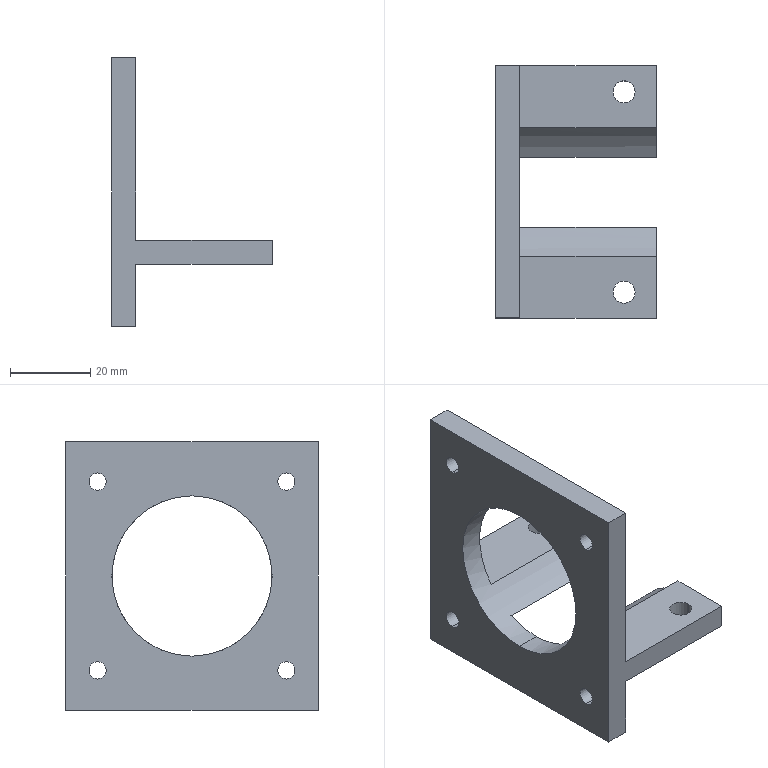Part | SolidWorks | features BaseBody 1 | 1 solid | 27 faces | box 40 x 63 x 67 mm | volume 24720 mm3 | cylinder 14 | plane 13 | commonest cylinder face diameters 4.3 x8 5.5 x4 40 x2
STEP:
#1=CARTESIAN_POINT('',(0.,-23.57,39.42));
#2=VERTEX_POINT('',#1);
#3=CARTESIAN_POINT('',(0.,-23.57,43.72));
#4=VERTEX_POINT('',#3);
#5=CARTESIAN_POINT('',(0.,-23.57,41.57));
#6=DIRECTION('',(-1.,0.,0.));
#7=DIRECTION('',(0.,0.,-1.));
#8=AXIS2_PLACEMENT_3D('',#5,#6,#7);
#9=CIRCLE('',#8,2.15);
#10=EDGE_CURVE('',#2,#4,#9,.T.);
#11=ORIENTED_EDGE('',*,*,#10,.T.);
#12=CARTESIAN_POINT('',(6.,-23.57,43.72));
#13=VERTEX_POINT('',#12);
#14=CARTESIAN_POINT('',(-6.2,-23.57,43.72));
#15=DIRECTION('',(1.,0.,0.));
#16=VECTOR('',#15,1000.);
#17=LINE('',#14,#16);
#18=EDGE_CURVE('',#4,#13,#17,.T.);
#19=ORIENTED_EDGE('',*,*,#18,.T.);
#20=CARTESIAN_POINT('',(6.,-23.57,39.42));
#21=VERTEX_POINT('',#20);
#22=CARTESIAN_POINT('',(6.,-23.57,41.57));
#23=DIRECTION('',(-1.,0.,0.));
#24=DIRECTION('',(0.,0.,-1.));
#25=AXIS2_PLACEMENT_3D('',#22,#23,#24);
#26=CIRCLE('',#25,2.15);
#27=EDGE_CURVE('',#21,#13,#26,.T.);
#28=ORIENTED_EDGE('',*,*,#27,.F.);
#29=CARTESIAN_POINT('',(-6.2,-23.57,39.42));
#30=DIRECTION('',(1.,0.,0.));
#31=VECTOR('',#30,1000.);
#32=LINE('',#29,#31);
#33=EDGE_CURVE('',#2,#21,#32,.T.);
#34=ORIENTED_EDGE('',*,*,#33,.F.);
#35=EDGE_LOOP('',(#11,#19,#28,#34));
#36=FACE_OUTER_BOUND('',#35,.T.);
#37=CARTESIAN_POINT('',(-6.2,-23.57,41.57));
#38=DIRECTION('',(1.,0.,0.));
#39=DIRECTION('',(0.,0.,-1.));
#40=AXIS2_PLACEMENT_3D('',#37,#38,#39);
#41=CYLINDRICAL_SURFACE('',#40,2.15);
#42=ADVANCED_FACE('',(#36),#41,.F.);
#43=CARTESIAN_POINT('',(0.,-23.57,-7.72));
#44=VERTEX_POINT('',#43);
#45=CARTESIAN_POINT('',(0.,-23.57,-3.42));
#46=VERTEX_POINT('',#45);
#47=CARTESIAN_POINT('',(0.,-23.57,-5.57));
#48=DIRECTION('',(-1.,0.,0.));
#49=DIRECTION('',(0.,0.,-1.));
#50=AXIS2_PLACEMENT_3D('',#47,#48,#49);
#51=CIRCLE('',#50,2.15);
#52=EDGE_CURVE('',#44,#46,#51,.T.);
#53=ORIENTED_EDGE('',*,*,#52,.T.);
#54=CARTESIAN_POINT('',(6.,-23.57,-3.42));
#55=VERTEX_POINT('',#54);
#56=CARTESIAN_POINT('',(-6.2,-23.57,-3.42));
#57=DIRECTION('',(1.,0.,0.));
#58=VECTOR('',#57,1000.);
#59=LINE('',#56,#58);
#60=EDGE_CURVE('',#46,#55,#59,.T.);
#61=ORIENTED_EDGE('',*,*,#60,.T.);
#62=CARTESIAN_POINT('',(6.,-23.57,-7.72));
#63=VERTEX_POINT('',#62);
#64=CARTESIAN_POINT('',(6.,-23.57,-5.57));
#65=DIRECTION('',(-1.,0.,0.));
#66=DIRECTION('',(0.,0.,-1.));
#67=AXIS2_PLACEMENT_3D('',#64,#65,#66);
#68=CIRCLE('',#67,2.15);
#69=EDGE_CURVE('',#63,#55,#68,.T.);
#70=ORIENTED_EDGE('',*,*,#69,.F.);
#71=CARTESIAN_POINT('',(-6.2,-23.57,-7.72));
#72=DIRECTION('',(1.,0.,0.));
#73=VECTOR('',#72,1000.);
#74=LINE('',#71,#73);
#75=EDGE_CURVE('',#44,#63,#74,.T.);
#76=ORIENTED_EDGE('',*,*,#75,.F.);
#77=EDGE_LOOP('',(#53,#61,#70,#76));
#78=FACE_OUTER_BOUND('',#77,.T.);
#79=CARTESIAN_POINT('',(-6.2,-23.57,-5.57));
#80=DIRECTION('',(1.,0.,0.));
#81=DIRECTION('',(0.,0.,-1.));
#82=AXIS2_PLACEMENT_3D('',#79,#80,#81);
#83=CYLINDRICAL_SURFACE('',#82,2.15);
#84=ADVANCED_FACE('',(#78),#83,.F.);
#85=CARTESIAN_POINT('',(0.,0.,-2.));
#86=VERTEX_POINT('',#85);
#87=CARTESIAN_POINT('',(0.,0.,38.));
#88=VERTEX_POINT('',#87);
#89=CARTESIAN_POINT('',(0.,0.,18.));
#90=DIRECTION('',(-1.,0.,0.));
#91=DIRECTION('',(0.,0.,-1.));
#92=AXIS2_PLACEMENT_3D('',#89,#90,#91);
#93=CIRCLE('',#92,20.);
#94=EDGE_CURVE('',#86,#88,#93,.T.);
#95=ORIENTED_EDGE('',*,*,#94,.T.);
#96=CARTESIAN_POINT('',(6.,0.,38.));
#97=VERTEX_POINT('',#96);
#98=CARTESIAN_POINT('',(-2.,0.,38.));
#99=DIRECTION('',(1.,0.,0.));
#100=VECTOR('',#99,1000.);
#101=LINE('',#98,#100);
#102=EDGE_CURVE('',#88,#97,#101,.T.);
#103=ORIENTED_EDGE('',*,*,#102,.T.);
#104=CARTESIAN_POINT('',(6.,-16.,6.));
#105=VERTEX_POINT('',#104);
#106=CARTESIAN_POINT('',(6.,0.,18.));
#107=DIRECTION('',(-1.,0.,0.));
#108=DIRECTION('',(0.,0.,-1.));
#109=AXIS2_PLACEMENT_3D('',#106,#107,#108);
#110=CIRCLE('',#109,20.);
#111=EDGE_CURVE('',#105,#97,#110,.T.);
#112=ORIENTED_EDGE('',*,*,#111,.F.);
#113=CARTESIAN_POINT('',(40.,-16.,6.));
#114=VERTEX_POINT('',#113);
#115=CARTESIAN_POINT('',(-2.,-16.,6.));
#116=DIRECTION('',(-1.,0.,0.));
#117=VECTOR('',#116,1000.);
#118=LINE('',#115,#117);
#119=EDGE_CURVE('',#114,#105,#118,.T.);
#120=ORIENTED_EDGE('',*,*,#119,.F.);
#121=CARTESIAN_POINT('',(40.,-8.718,0.));
#122=VERTEX_POINT('',#121);
#123=CARTESIAN_POINT('',(40.,0.,18.));
#124=DIRECTION('',(-1.,0.,0.));
#125=DIRECTION('',(0.,0.,-1.));
#126=AXIS2_PLACEMENT_3D('',#123,#124,#125);
#127=CIRCLE('',#126,20.);
#128=EDGE_CURVE('',#122,#114,#127,.T.);
#129=ORIENTED_EDGE('',*,*,#128,.F.);
#130=CARTESIAN_POINT('',(6.,-8.718,0.));
#131=VERTEX_POINT('',#130);
#132=CARTESIAN_POINT('',(-2.,-8.718,0.));
#133=DIRECTION('',(1.,0.,0.));
#134=VECTOR('',#133,1000.);
#135=LINE('',#132,#134);
#136=EDGE_CURVE('',#131,#122,#135,.T.);
#137=ORIENTED_EDGE('',*,*,#136,.F.);
#138=CARTESIAN_POINT('',(6.,0.,-2.));
#139=VERTEX_POINT('',#138);
#140=CARTESIAN_POINT('',(6.,0.,18.));
#141=DIRECTION('',(-1.,0.,0.));
#142=DIRECTION('',(0.,0.,-1.));
#143=AXIS2_PLACEMENT_3D('',#140,#141,#142);
#144=CIRCLE('',#143,20.);
#145=EDGE_CURVE('',#139,#131,#144,.T.);
#146=ORIENTED_EDGE('',*,*,#145,.F.);
#147=CARTESIAN_POINT('',(-2.,0.,-2.));
#148=DIRECTION('',(1.,0.,0.));
#149=VECTOR('',#148,1000.);
#150=LINE('',#147,#149);
#151=EDGE_CURVE('',#86,#139,#150,.T.);
#152=ORIENTED_EDGE('',*,*,#151,.F.);
#153=EDGE_LOOP('',(#95,#103,#112,#120,#129,#137,#146,#152));
#154=FACE_OUTER_BOUND('',#153,.T.);
#155=CARTESIAN_POINT('',(-2.,0.,18.));
#156=DIRECTION('',(1.,0.,0.));
#157=DIRECTION('',(0.,0.,-1.));
#158=AXIS2_PLACEMENT_3D('',#155,#156,#157);
#159=CYLINDRICAL_SURFACE('',#158,20.);
#160=ADVANCED_FACE('',(#154),#159,.F.);
#161=CARTESIAN_POINT('',(0.,23.57,39.42));
#162=VERTEX_POINT('',#161);
#163=CARTESIAN_POINT('',(0.,23.57,43.72));
#164=VERTEX_POINT('',#163);
#165=CARTESIAN_POINT('',(0.,23.57,41.57));
#166=DIRECTION('',(-1.,0.,0.));
#167=DIRECTION('',(0.,0.,-1.));
#168=AXIS2_PLACEMENT_3D('',#165,#166,#167);
#169=CIRCLE('',#168,2.15);
#170=EDGE_CURVE('',#162,#164,#169,.T.);
#171=ORIENTED_EDGE('',*,*,#170,.T.);
#172=CARTESIAN_POINT('',(6.,23.57,43.72));
#173=VERTEX_POINT('',#172);
#174=CARTESIAN_POINT('',(-6.2,23.57,43.72));
#175=DIRECTION('',(1.,0.,0.));
#176=VECTOR('',#175,1000.);
#177=LINE('',#174,#176);
#178=EDGE_CURVE('',#164,#173,#177,.T.);
#179=ORIENTED_EDGE('',*,*,#178,.T.);
#180=CARTESIAN_POINT('',(6.,23.57,39.42));
#181=VERTEX_POINT('',#180);
#182=CARTESIAN_POINT('',(6.,23.57,41.57));
#183=DIRECTION('',(-1.,0.,0.));
#184=DIRECTION('',(0.,0.,-1.));
#185=AXIS2_PLACEMENT_3D('',#182,#183,#184);
#186=CIRCLE('',#185,2.15);
#187=EDGE_CURVE('',#181,#173,#186,.T.);
#188=ORIENTED_EDGE('',*,*,#187,.F.);
#189=CARTESIAN_POINT('',(-6.2,23.57,39.42));
#190=DIRECTION('',(1.,0.,0.));
#191=VECTOR('',#190,1000.);
#192=LINE('',#189,#191);
#193=EDGE_CURVE('',#162,#181,#192,.T.);
#194=ORIENTED_EDGE('',*,*,#193,.F.);
#195=EDGE_LOOP('',(#171,#179,#188,#194));
#196=FACE_OUTER_BOUND('',#195,.T.);
#197=CARTESIAN_POINT('',(-6.2,23.57,41.57));
#198=DIRECTION('',(1.,0.,0.));
#199=DIRECTION('',(0.,0.,-1.));
#200=AXIS2_PLACEMENT_3D('',#197,#198,#199);
#201=CYLINDRICAL_SURFACE('',#200,2.15);
#202=ADVANCED_FACE('',(#196),#201,.F.);
#203=CARTESIAN_POINT('',(0.,23.57,-7.72));
#204=VERTEX_POINT('',#203);
#205=CARTESIAN_POINT('',(0.,23.57,-3.42));
#206=VERTEX_POINT('',#205);
#207=CARTESIAN_POINT('',(0.,23.57,-5.57));
#208=DIRECTION('',(-1.,0.,0.));
#209=DIRECTION('',(0.,0.,-1.));
#210=AXIS2_PLACEMENT_3D('',#207,#208,#209);
#211=CIRCLE('',#210,2.15);
#212=EDGE_CURVE('',#204,#206,#211,.T.);
#213=ORIENTED_EDGE('',*,*,#212,.T.);
#214=CARTESIAN_POINT('',(6.,23.57,-3.42));
#215=VERTEX_POINT('',#214);
#216=CARTESIAN_POINT('',(-6.2,23.57,-3.42));
#217=DIRECTION('',(1.,0.,0.));
#218=VECTOR('',#217,1000.);
#219=LINE('',#216,#218);
#220=EDGE_CURVE('',#206,#215,#219,.T.);
#221=ORIENTED_EDGE('',*,*,#220,.T.);
#222=CARTESIAN_POINT('',(6.,23.57,-7.72));
#223=VERTEX_POINT('',#222);
#224=CARTESIAN_POINT('',(6.,23.57,-5.57));
#225=DIRECTION('',(-1.,0.,0.));
#226=DIRECTION('',(0.,0.,-1.));
#227=AXIS2_PLACEMENT_3D('',#224,#225,#226);
#228=CIRCLE('',#227,2.15);
#229=EDGE_CURVE('',#223,#215,#228,.T.);
#230=ORIENTED_EDGE('',*,*,#229,.F.);
#231=CARTESIAN_POINT('',(-6.2,23.57,-7.72));
#232=DIRECTION('',(1.,0.,0.));
#233=VECTOR('',#232,1000.);
#234=LINE('',#231,#233);
#235=EDGE_CURVE('',#204,#223,#234,.T.);
#236=ORIENTED_EDGE('',*,*,#235,.F.);
#237=EDGE_LOOP('',(#213,#221,#230,#236));
#238=FACE_OUTER_BOUND('',#237,.T.);
#239=CARTESIAN_POINT('',(-6.2,23.57,-5.57));
#240=DIRECTION('',(1.,0.,0.));
#241=DIRECTION('',(0.,0.,-1.));
#242=AXIS2_PLACEMENT_3D('',#239,#240,#241);
#243=CYLINDRICAL_SURFACE('',#242,2.15);
#244=ADVANCED_FACE('',(#238),#243,.F.);
#245=CARTESIAN_POINT('',(34.75,25.,0.));
#246=VERTEX_POINT('',#245);
#247=CARTESIAN_POINT('',(29.25,25.,0.));
#248=VERTEX_POINT('',#247);
#249=CARTESIAN_POINT('',(32.,25.,0.));
#250=DIRECTION('',(0.,0.,-1.));
#251=DIRECTION('',(1.,0.,0.));
#252=AXIS2_PLACEMENT_3D('',#249,#250,#251);
#253=CIRCLE('',#252,2.75);
#254=EDGE_CURVE('',#246,#248,#253,.T.);
#255=ORIENTED_EDGE('',*,*,#254,.T.);
#256=CARTESIAN_POINT('',(29.25,25.,6.));
#257=VERTEX_POINT('',#256);
#258=CARTESIAN_POINT('',(29.25,25.,-1.));
#259=DIRECTION('',(0.,0.,1.));
#260=VECTOR('',#259,1000.);
#261=LINE('',#258,#260);
#262=EDGE_CURVE('',#248,#257,#261,.T.);
#263=ORIENTED_EDGE('',*,*,#262,.T.);
#264=CARTESIAN_POINT('',(34.75,25.,6.));
#265=VERTEX_POINT('',#264);
#266=CARTESIAN_POINT('',(32.,25.,6.));
#267=DIRECTION('',(0.,0.,-1.));
#268=DIRECTION('',(1.,0.,0.));
#269=AXIS2_PLACEMENT_3D('',#266,#267,#268);
#270=CIRCLE('',#269,2.75);
#271=EDGE_CURVE('',#265,#257,#270,.T.);
#272=ORIENTED_EDGE('',*,*,#271,.F.);
#273=CARTESIAN_POINT('',(34.75,25.,-1.));
#274=DIRECTION('',(0.,0.,1.));
#275=VECTOR('',#274,1000.);
#276=LINE('',#273,#275);
#277=EDGE_CURVE('',#246,#265,#276,.T.);
#278=ORIENTED_EDGE('',*,*,#277,.F.);
#279=EDGE_LOOP('',(#255,#263,#272,#278));
#280=FACE_OUTER_BOUND('',#279,.T.);
#281=CARTESIAN_POINT('',(32.,25.,-1.));
#282=DIRECTION('',(0.,0.,1.));
#283=DIRECTION('',(1.,0.,0.));
#284=AXIS2_PLACEMENT_3D('',#281,#282,#283);
#285=CYLINDRICAL_SURFACE('',#284,2.75);
#286=ADVANCED_FACE('',(#280),#285,.F.);
#287=CARTESIAN_POINT('',(34.75,-25.,0.));
#288=VERTEX_POINT('',#287);
#289=CARTESIAN_POINT('',(29.25,-25.,0.));
#290=VERTEX_POINT('',#289);
#291=CARTESIAN_POINT('',(32.,-25.,0.));
#292=DIRECTION('',(0.,0.,-1.));
#293=DIRECTION('',(1.,0.,0.));
#294=AXIS2_PLACEMENT_3D('',#291,#292,#293);
#295=CIRCLE('',#294,2.75);
#296=EDGE_CURVE('',#288,#290,#295,.T.);
#297=ORIENTED_EDGE('',*,*,#296,.T.);
#298=CARTESIAN_POINT('',(29.25,-25.,6.));
#299=VERTEX_POINT('',#298);
#300=CARTESIAN_POINT('',(29.25,-25.,-1.));
#301=DIRECTION('',(0.,0.,1.));
#302=VECTOR('',#301,1000.);
#303=LINE('',#300,#302);
#304=EDGE_CURVE('',#290,#299,#303,.T.);
#305=ORIENTED_EDGE('',*,*,#304,.T.);
#306=CARTESIAN_POINT('',(34.75,-25.,6.));
#307=VERTEX_POINT('',#306);
#308=CARTESIAN_POINT('',(32.,-25.,6.));
#309=DIRECTION('',(0.,0.,-1.));
#310=DIRECTION('',(1.,0.,0.));
#311=AXIS2_PLACEMENT_3D('',#308,#309,#310);
#312=CIRCLE('',#311,2.75);
#313=EDGE_CURVE('',#307,#299,#312,.T.);
#314=ORIENTED_EDGE('',*,*,#313,.F.);
#315=CARTESIAN_POINT('',(34.75,-25.,-1.));
#316=DIRECTION('',(0.,0.,1.));
#317=VECTOR('',#316,1000.);
#318=LINE('',#315,#317);
#319=EDGE_CURVE('',#288,#307,#318,.T.);
#320=ORIENTED_EDGE('',*,*,#319,.F.);
#321=EDGE_LOOP('',(#297,#305,#314,#320));
#322=FACE_OUTER_BOUND('',#321,.T.);
#323=CARTESIAN_POINT('',(32.,-25.,-1.));
#324=DIRECTION('',(0.,0.,1.));
#325=DIRECTION('',(1.,0.,0.));
#326=AXIS2_PLACEMENT_3D('',#323,#324,#325);
#327=CYLINDRICAL_SURFACE('',#326,2.75);
#328=ADVANCED_FACE('',(#322),#327,.F.);
#329=ORIENTED_EDGE('',*,*,#10,.F.);
#330=CARTESIAN_POINT('',(0.,-23.57,41.57));
#331=DIRECTION('',(-1.,0.,0.));
#332=DIRECTION('',(0.,0.,-1.));
#333=AXIS2_PLACEMENT_3D('',#330,#331,#332);
#334=CIRCLE('',#333,2.15);
#335=EDGE_CURVE('',#4,#2,#334,.T.);
#336=ORIENTED_EDGE('',*,*,#335,.F.);
#337=EDGE_LOOP('',(#329,#336));
#338=FACE_BOUND('',#337,.T.);
#339=ORIENTED_EDGE('',*,*,#52,.F.);
#340=CARTESIAN_POINT('',(0.,-23.57,-5.57));
#341=DIRECTION('',(-1.,0.,0.));
#342=DIRECTION('',(0.,0.,-1.));
#343=AXIS2_PLACEMENT_3D('',#340,#341,#342);
#344=CIRCLE('',#343,2.15);
#345=EDGE_CURVE('',#46,#44,#344,.T.);
#346=ORIENTED_EDGE('',*,*,#345,.F.);
#347=EDGE_LOOP('',(#339,#346));
#348=FACE_BOUND('',#347,.T.);
#349=ORIENTED_EDGE('',*,*,#94,.F.);
#350=CARTESIAN_POINT('',(0.,0.,18.));
#351=DIRECTION('',(-1.,0.,0.));
#352=DIRECTION('',(0.,0.,-1.));
#353=AXIS2_PLACEMENT_3D('',#350,#351,#352);
#354=CIRCLE('',#353,20.);
#355=EDGE_CURVE('',#88,#86,#354,.T.);
#356=ORIENTED_EDGE('',*,*,#355,.F.);
#357=EDGE_LOOP('',(#349,#356));
#358=FACE_BOUND('',#357,.T.);
#359=ORIENTED_EDGE('',*,*,#170,.F.);
#360=CARTESIAN_POINT('',(0.,23.57,41.57));
#361=DIRECTION('',(-1.,0.,0.));
#362=DIRECTION('',(0.,0.,-1.));
#363=AXIS2_PLACEMENT_3D('',#360,#361,#362);
#364=CIRCLE('',#363,2.15);
#365=EDGE_CURVE('',#164,#162,#364,.T.);
#366=ORIENTED_EDGE('',*,*,#365,.F.);
#367=EDGE_LOOP('',(#359,#366));
#368=FACE_BOUND('',#367,.T.);
#369=ORIENTED_EDGE('',*,*,#212,.F.);
#370=CARTESIAN_POINT('',(0.,23.57,-5.57));
#371=DIRECTION('',(-1.,0.,0.));
#372=DIRECTION('',(0.,0.,-1.));
#373=AXIS2_PLACEMENT_3D('',#370,#371,#372);
#374=CIRCLE('',#373,2.15);
#375=EDGE_CURVE('',#206,#204,#374,.T.);
#376=ORIENTED_EDGE('',*,*,#375,.F.);
#377=EDGE_LOOP('',(#369,#376));
#378=FACE_BOUND('',#377,.T.);
#379=CARTESIAN_POINT('',(0.,31.5,-15.5));
#380=VERTEX_POINT('',#379);
#381=CARTESIAN_POINT('',(0.,31.5,51.5));
#382=VERTEX_POINT('',#381);
#383=CARTESIAN_POINT('',(0.,31.5,-15.5));
#384=DIRECTION('',(0.,0.,1.));
#385=VECTOR('',#384,1000.);
#386=LINE('',#383,#385);
#387=EDGE_CURVE('',#380,#382,#386,.T.);
#388=ORIENTED_EDGE('',*,*,#387,.F.);
#389=CARTESIAN_POINT('',(0.,-31.5,-15.5));
#390=VERTEX_POINT('',#389);
#391=CARTESIAN_POINT('',(0.,-31.5,-15.5));
#392=DIRECTION('',(0.,1.,0.));
#393=VECTOR('',#392,1000.);
#394=LINE('',#391,#393);
#395=EDGE_CURVE('',#390,#380,#394,.T.);
#396=ORIENTED_EDGE('',*,*,#395,.F.);
#397=CARTESIAN_POINT('',(0.,-31.5,51.5));
#398=VERTEX_POINT('',#397);
#399=CARTESIAN_POINT('',(0.,-31.5,-15.5));
#400=DIRECTION('',(0.,0.,-1.));
#401=VECTOR('',#400,1000.);
#402=LINE('',#399,#401);
#403=EDGE_CURVE('',#398,#390,#402,.T.);
#404=ORIENTED_EDGE('',*,*,#403,.F.);
#405=CARTESIAN_POINT('',(0.,-31.5,51.5));
#406=DIRECTION('',(0.,-1.,0.));
#407=VECTOR('',#406,1000.);
#408=LINE('',#405,#407);
#409=EDGE_CURVE('',#382,#398,#408,.T.);
#410=ORIENTED_EDGE('',*,*,#409,.F.);
#411=EDGE_LOOP('',(#388,#396,#404,#410));
#412=FACE_OUTER_BOUND('',#411,.T.);
#413=CARTESIAN_POINT('',(0.,-31.5,-15.5));
#414=DIRECTION('',(1.,0.,0.));
#415=DIRECTION('',(0.,0.,-1.));
#416=AXIS2_PLACEMENT_3D('',#413,#414,#415);
#417=PLANE('',#416);
#418=ADVANCED_FACE('',(#338,#348,#358,#368,#378,#412),#417,.F.);
#419=ORIENTED_EDGE('',*,*,#18,.F.);
#420=ORIENTED_EDGE('',*,*,#335,.T.);
#421=ORIENTED_EDGE('',*,*,#33,.T.);
#422=CARTESIAN_POINT('',(6.,-23.57,41.57));
#423=DIRECTION('',(-1.,0.,0.));
#424=DIRECTION('',(0.,0.,-1.));
#425=AXIS2_PLACEMENT_3D('',#422,#423,#424);
#426=CIRCLE('',#425,2.15);
#427=EDGE_CURVE('',#13,#21,#426,.T.);
#428=ORIENTED_EDGE('',*,*,#427,.F.);
#429=EDGE_LOOP('',(#419,#420,#421,#428));
#430=FACE_OUTER_BOUND('',#429,.T.);
#431=CARTESIAN_POINT('',(-6.2,-23.57,41.57));
#432=DIRECTION('',(1.,0.,0.));
#433=DIRECTION('',(0.,0.,-1.));
#434=AXIS2_PLACEMENT_3D('',#431,#432,#433);
#435=CYLINDRICAL_SURFACE('',#434,2.15);
#436=ADVANCED_FACE('',(#430),#435,.F.);
#437=ORIENTED_EDGE('',*,*,#60,.F.);
#438=ORIENTED_EDGE('',*,*,#345,.T.);
#439=ORIENTED_EDGE('',*,*,#75,.T.);
#440=CARTESIAN_POINT('',(6.,-23.57,-5.57));
#441=DIRECTION('',(-1.,0.,0.));
#442=DIRECTION('',(0.,0.,-1.));
#443=AXIS2_PLACEMENT_3D('',#440,#441,#442);
#444=CIRCLE('',#443,2.15);
#445=EDGE_CURVE('',#55,#63,#444,.T.);
#446=ORIENTED_EDGE('',*,*,#445,.F.);
#447=EDGE_LOOP('',(#437,#438,#439,#446));
#448=FACE_OUTER_BOUND('',#447,.T.);
#449=CARTESIAN_POINT('',(-6.2,-23.57,-5.57));
#450=DIRECTION('',(1.,0.,0.));
#451=DIRECTION('',(0.,0.,-1.));
#452=AXIS2_PLACEMENT_3D('',#449,#450,#451);
#453=CYLINDRICAL_SURFACE('',#452,2.15);
#454=ADVANCED_FACE('',(#448),#453,.F.);
#455=ORIENTED_EDGE('',*,*,#102,.F.);
#456=ORIENTED_EDGE('',*,*,#355,.T.);
#457=ORIENTED_EDGE('',*,*,#151,.T.);
#458=CARTESIAN_POINT('',(6.,8.718,0.));
#459=VERTEX_POINT('',#458);
#460=CARTESIAN_POINT('',(6.,0.,18.));
#461=DIRECTION('',(-1.,0.,0.));
#462=DIRECTION('',(0.,0.,-1.));
#463=AXIS2_PLACEMENT_3D('',#460,#461,#462);
#464=CIRCLE('',#463,20.);
#465=EDGE_CURVE('',#459,#139,#464,.T.);
#466=ORIENTED_EDGE('',*,*,#465,.F.);
#467=CARTESIAN_POINT('',(40.,8.718,0.));
#468=VERTEX_POINT('',#467);
#469=CARTESIAN_POINT('',(-2.,8.718,0.));
#470=DIRECTION('',(-1.,0.,0.));
#471=VECTOR('',#470,1000.);
#472=LINE('',#469,#471);
#473=EDGE_CURVE('',#468,#459,#472,.T.);
#474=ORIENTED_EDGE('',*,*,#473,.F.);
#475=CARTESIAN_POINT('',(40.,16.,6.));
#476=VERTEX_POINT('',#475);
#477=CARTESIAN_POINT('',(40.,0.,18.));
#478=DIRECTION('',(-1.,0.,0.));
#479=DIRECTION('',(0.,0.,-1.));
#480=AXIS2_PLACEMENT_3D('',#477,#478,#479);
#481=CIRCLE('',#480,20.);
#482=EDGE_CURVE('',#476,#468,#481,.T.);
#483=ORIENTED_EDGE('',*,*,#482,.F.);
#484=CARTESIAN_POINT('',(6.,16.,6.));
#485=VERTEX_POINT('',#484);
#486=CARTESIAN_POINT('',(-2.,16.,6.));
#487=DIRECTION('',(1.,0.,0.));
#488=VECTOR('',#487,1000.);
#489=LINE('',#486,#488);
#490=EDGE_CURVE('',#485,#476,#489,.T.);
#491=ORIENTED_EDGE('',*,*,#490,.F.);
#492=CARTESIAN_POINT('',(6.,0.,18.));
#493=DIRECTION('',(-1.,0.,0.));
#494=DIRECTION('',(0.,0.,-1.));
#495=AXIS2_PLACEMENT_3D('',#492,#493,#494);
#496=CIRCLE('',#495,20.);
#497=EDGE_CURVE('',#97,#485,#496,.T.);
#498=ORIENTED_EDGE('',*,*,#497,.F.);
#499=EDGE_LOOP('',(#455,#456,#457,#466,#474,#483,#491,#498));
#500=FACE_OUTER_BOUND('',#499,.T.);
#501=CARTESIAN_POINT('',(-2.,0.,18.));
#502=DIRECTION('',(1.,0.,0.));
#503=DIRECTION('',(0.,0.,-1.));
#504=AXIS2_PLACEMENT_3D('',#501,#502,#503);
#505=CYLINDRICAL_SURFACE('',#504,20.);
#506=ADVANCED_FACE('',(#500),#505,.F.);
#507=ORIENTED_EDGE('',*,*,#178,.F.);
#508=ORIENTED_EDGE('',*,*,#365,.T.);
#509=ORIENTED_EDGE('',*,*,#193,.T.);
#510=CARTESIAN_POINT('',(6.,23.57,41.57));
#511=DIRECTION('',(-1.,0.,0.));
#512=DIRECTION('',(0.,0.,-1.));
#513=AXIS2_PLACEMENT_3D('',#510,#511,#512);
#514=CIRCLE('',#513,2.15);
#515=EDGE_CURVE('',#173,#181,#514,.T.);
#516=ORIENTED_EDGE('',*,*,#515,.F.);
#517=EDGE_LOOP('',(#507,#508,#509,#516));
#518=FACE_OUTER_BOUND('',#517,.T.);
#519=CARTESIAN_POINT('',(-6.2,23.57,41.57));
#520=DIRECTION('',(1.,0.,0.));
#521=DIRECTION('',(0.,0.,-1.));
#522=AXIS2_PLACEMENT_3D('',#519,#520,#521);
#523=CYLINDRICAL_SURFACE('',#522,2.15);
#524=ADVANCED_FACE('',(#518),#523,.F.);
#525=ORIENTED_EDGE('',*,*,#220,.F.);
#526=ORIENTED_EDGE('',*,*,#375,.T.);
#527=ORIENTED_EDGE('',*,*,#235,.T.);
#528=CARTESIAN_POINT('',(6.,23.57,-5.57));
#529=DIRECTION('',(-1.,0.,0.));
#530=DIRECTION('',(0.,0.,-1.));
#531=AXIS2_PLACEMENT_3D('',#528,#529,#530);
#532=CIRCLE('',#531,2.15);
#533=EDGE_CURVE('',#215,#223,#532,.T.);
#534=ORIENTED_EDGE('',*,*,#533,.F.);
#535=EDGE_LOOP('',(#525,#526,#527,#534));
#536=FACE_OUTER_BOUND('',#535,.T.);
#537=CARTESIAN_POINT('',(-6.2,23.57,-5.57));
#538=DIRECTION('',(1.,0.,0.));
#539=DIRECTION('',(0.,0.,-1.));
#540=AXIS2_PLACEMENT_3D('',#537,#538,#539);
#541=CYLINDRICAL_SURFACE('',#540,2.15);
#542=ADVANCED_FACE('',(#536),#541,.F.);
#543=CARTESIAN_POINT('',(6.,-31.5,51.5));
#544=VERTEX_POINT('',#543);
#545=CARTESIAN_POINT('',(6.,31.5,51.5));
#546=VERTEX_POINT('',#545);
#547=CARTESIAN_POINT('',(6.,-31.5,51.5));
#548=DIRECTION('',(0.,1.,0.));
#549=VECTOR('',#548,1000.);
#550=LINE('',#547,#549);
#551=EDGE_CURVE('',#544,#546,#550,.T.);
#552=ORIENTED_EDGE('',*,*,#551,.T.);
#553=CARTESIAN_POINT('',(0.,31.5,51.5));
#554=DIRECTION('',(-1.,0.,0.));
#555=VECTOR('',#554,1000.);
#556=LINE('',#553,#555);
#557=EDGE_CURVE('',#546,#382,#556,.T.);
#558=ORIENTED_EDGE('',*,*,#557,.T.);
#559=ORIENTED_EDGE('',*,*,#409,.T.);
#560=CARTESIAN_POINT('',(0.,-31.5,51.5));
#561=DIRECTION('',(1.,0.,0.));
#562=VECTOR('',#561,1000.);
#563=LINE('',#560,#562);
#564=EDGE_CURVE('',#398,#544,#563,.T.);
#565=ORIENTED_EDGE('',*,*,#564,.T.);
#566=EDGE_LOOP('',(#552,#558,#559,#565));
#567=FACE_OUTER_BOUND('',#566,.T.);
#568=CARTESIAN_POINT('',(0.,-31.5,51.5));
#569=DIRECTION('',(0.,0.,1.));
#570=DIRECTION('',(1.,0.,0.));
#571=AXIS2_PLACEMENT_3D('',#568,#569,#570);
#572=PLANE('',#571);
#573=ADVANCED_FACE('',(#567),#572,.T.);
#574=CARTESIAN_POINT('',(40.,31.5,6.));
#575=VERTEX_POINT('',#574);
#576=CARTESIAN_POINT('',(40.,31.5,0.));
#577=VERTEX_POINT('',#576);
#578=CARTESIAN_POINT('',(40.,31.5,-15.5));
#579=DIRECTION('',(0.,0.,-1.));
#580=VECTOR('',#579,1000.);
#581=LINE('',#578,#580);
#582=EDGE_CURVE('',#575,#577,#581,.T.);
#583=ORIENTED_EDGE('',*,*,#582,.T.);
#584=CARTESIAN_POINT('',(6.,31.5,0.));
#585=VERTEX_POINT('',#584);
#586=CARTESIAN_POINT('',(0.,31.5,0.));
#587=DIRECTION('',(-1.,0.,0.));
#588=VECTOR('',#587,1000.);
#589=LINE('',#586,#588);
#590=EDGE_CURVE('',#577,#585,#589,.T.);
#591=ORIENTED_EDGE('',*,*,#590,.T.);
#592=CARTESIAN_POINT('',(6.,31.5,-15.5));
#593=VERTEX_POINT('',#592);
#594=CARTESIAN_POINT('',(6.,31.5,-15.5));
#595=DIRECTION('',(0.,0.,-1.));
#596=VECTOR('',#595,1000.);
#597=LINE('',#594,#596);
#598=EDGE_CURVE('',#585,#593,#597,.T.);
#599=ORIENTED_EDGE('',*,*,#598,.T.);
#600=CARTESIAN_POINT('',(0.,31.5,-15.5));
#601=DIRECTION('',(-1.,0.,0.));
#602=VECTOR('',#601,1000.);
#603=LINE('',#600,#602);
#604=EDGE_CURVE('',#593,#380,#603,.T.);
#605=ORIENTED_EDGE('',*,*,#604,.T.);
#606=ORIENTED_EDGE('',*,*,#387,.T.);
#607=ORIENTED_EDGE('',*,*,#557,.F.);
#608=CARTESIAN_POINT('',(6.,31.5,6.));
#609=VERTEX_POINT('',#608);
#610=CARTESIAN_POINT('',(6.,31.5,-15.5));
#611=DIRECTION('',(0.,0.,-1.));
#612=VECTOR('',#611,1000.);
#613=LINE('',#610,#612);
#614=EDGE_CURVE('',#546,#609,#613,.T.);
#615=ORIENTED_EDGE('',*,*,#614,.T.);
#616=CARTESIAN_POINT('',(0.,31.5,6.));
#617=DIRECTION('',(1.,0.,0.));
#618=VECTOR('',#617,1000.);
#619=LINE('',#616,#618);
#620=EDGE_CURVE('',#609,#575,#619,.T.);
#621=ORIENTED_EDGE('',*,*,#620,.T.);
#622=EDGE_LOOP('',(#583,#591,#599,#605,#606,#607,#615,#621));
#623=FACE_OUTER_BOUND('',#622,.T.);
#624=CARTESIAN_POINT('',(0.,31.5,-15.5));
#625=DIRECTION('',(0.,1.,0.));
#626=DIRECTION('',(0.,0.,1.));
#627=AXIS2_PLACEMENT_3D('',#624,#625,#626);
#628=PLANE('',#627);
#629=ADVANCED_FACE('',(#623),#628,.T.);
#630=CARTESIAN_POINT('',(6.,-31.5,-15.5));
#631=VERTEX_POINT('',#630);
#632=CARTESIAN_POINT('',(6.,-31.5,-15.5));
#633=DIRECTION('',(0.,1.,0.));
#634=VECTOR('',#633,1000.);
#635=LINE('',#632,#634);
#636=EDGE_CURVE('',#631,#593,#635,.T.);
#637=ORIENTED_EDGE('',*,*,#636,.F.);
#638=CARTESIAN_POINT('',(0.,-31.5,-15.5));
#639=DIRECTION('',(1.,0.,0.));
#640=VECTOR('',#639,1000.);
#641=LINE('',#638,#640);
#642=EDGE_CURVE('',#390,#631,#641,.T.);
#643=ORIENTED_EDGE('',*,*,#642,.F.);
#644=ORIENTED_EDGE('',*,*,#395,.T.);
#645=ORIENTED_EDGE('',*,*,#604,.F.);
#646=EDGE_LOOP('',(#637,#643,#644,#645));
#647=FACE_OUTER_BOUND('',#646,.T.);
#648=CARTESIAN_POINT('',(0.,-31.5,-15.5));
#649=DIRECTION('',(0.,0.,1.));
#650=DIRECTION('',(1.,0.,0.));
#651=AXIS2_PLACEMENT_3D('',#648,#649,#650);
#652=PLANE('',#651);
#653=ADVANCED_FACE('',(#647),#652,.F.);
#654=CARTESIAN_POINT('',(40.,-31.5,6.));
#655=VERTEX_POINT('',#654);
#656=CARTESIAN_POINT('',(40.,-31.5,0.));
#657=VERTEX_POINT('',#656);
#658=CARTESIAN_POINT('',(40.,-31.5,-15.5));
#659=DIRECTION('',(0.,0.,-1.));
#660=VECTOR('',#659,1000.);
#661=LINE('',#658,#660);
#662=EDGE_CURVE('',#655,#657,#661,.T.);
#663=ORIENTED_EDGE('',*,*,#662,.F.);
#664=CARTESIAN_POINT('',(6.,-31.5,6.));
#665=VERTEX_POINT('',#664);
#666=CARTESIAN_POINT('',(0.,-31.5,6.));
#667=DIRECTION('',(1.,0.,0.));
#668=VECTOR('',#667,1000.);
#669=LINE('',#666,#668);
#670=EDGE_CURVE('',#665,#655,#669,.T.);
#671=ORIENTED_EDGE('',*,*,#670,.F.);
#672=CARTESIAN_POINT('',(6.,-31.5,-15.5));
#673=DIRECTION('',(0.,0.,-1.));
#674=VECTOR('',#673,1000.);
#675=LINE('',#672,#674);
#676=EDGE_CURVE('',#544,#665,#675,.T.);
#677=ORIENTED_EDGE('',*,*,#676,.F.);
#678=ORIENTED_EDGE('',*,*,#564,.F.);
#679=ORIENTED_EDGE('',*,*,#403,.T.);
#680=ORIENTED_EDGE('',*,*,#642,.T.);
#681=CARTESIAN_POINT('',(6.,-31.5,0.));
#682=VERTEX_POINT('',#681);
#683=CARTESIAN_POINT('',(6.,-31.5,-15.5));
#684=DIRECTION('',(0.,0.,-1.));
#685=VECTOR('',#684,1000.);
#686=LINE('',#683,#685);
#687=EDGE_CURVE('',#682,#631,#686,.T.);
#688=ORIENTED_EDGE('',*,*,#687,.F.);
#689=CARTESIAN_POINT('',(0.,-31.5,0.));
#690=DIRECTION('',(-1.,0.,0.));
#691=VECTOR('',#690,1000.);
#692=LINE('',#689,#691);
#693=EDGE_CURVE('',#657,#682,#692,.T.);
#694=ORIENTED_EDGE('',*,*,#693,.F.);
#695=EDGE_LOOP('',(#663,#671,#677,#678,#679,#680,#688,#694));
#696=FACE_OUTER_BOUND('',#695,.T.);
#697=CARTESIAN_POINT('',(0.,-31.5,-15.5));
#698=DIRECTION('',(0.,1.,0.));
#699=DIRECTION('',(0.,0.,1.));
#700=AXIS2_PLACEMENT_3D('',#697,#698,#699);
#701=PLANE('',#700);
#702=ADVANCED_FACE('',(#696),#701,.F.);
#703=ORIENTED_EDGE('',*,*,#27,.T.);
#704=ORIENTED_EDGE('',*,*,#427,.T.);
#705=EDGE_LOOP('',(#703,#704));
#706=FACE_BOUND('',#705,.T.);
#707=ORIENTED_EDGE('',*,*,#187,.T.);
#708=ORIENTED_EDGE('',*,*,#515,.T.);
#709=EDGE_LOOP('',(#707,#708));
#710=FACE_BOUND('',#709,.T.);
#711=ORIENTED_EDGE('',*,*,#614,.F.);
#712=ORIENTED_EDGE('',*,*,#551,.F.);
#713=ORIENTED_EDGE('',*,*,#676,.T.);
#714=CARTESIAN_POINT('',(6.,-31.5,6.));
#715=DIRECTION('',(0.,1.,0.));
#716=VECTOR('',#715,1000.);
#717=LINE('',#714,#716);
#718=EDGE_CURVE('',#665,#105,#717,.T.);
#719=ORIENTED_EDGE('',*,*,#718,.T.);
#720=ORIENTED_EDGE('',*,*,#111,.T.);
#721=ORIENTED_EDGE('',*,*,#497,.T.);
#722=CARTESIAN_POINT('',(6.,-31.5,6.));
#723=DIRECTION('',(0.,1.,0.));
#724=VECTOR('',#723,1000.);
#725=LINE('',#722,#724);
#726=EDGE_CURVE('',#485,#609,#725,.T.);
#727=ORIENTED_EDGE('',*,*,#726,.T.);
#728=EDGE_LOOP('',(#711,#712,#713,#719,#720,#721,#727));
#729=FACE_OUTER_BOUND('',#728,.T.);
#730=CARTESIAN_POINT('',(6.,-31.5,-15.5));
#731=DIRECTION('',(1.,0.,0.));
#732=DIRECTION('',(0.,0.,-1.));
#733=AXIS2_PLACEMENT_3D('',#730,#731,#732);
#734=PLANE('',#733);
#735=ADVANCED_FACE('',(#706,#710,#729),#734,.T.);
#736=ORIENTED_EDGE('',*,*,#69,.T.);
#737=ORIENTED_EDGE('',*,*,#445,.T.);
#738=EDGE_LOOP('',(#736,#737));
#739=FACE_BOUND('',#738,.T.);
#740=ORIENTED_EDGE('',*,*,#229,.T.);
#741=ORIENTED_EDGE('',*,*,#533,.T.);
#742=EDGE_LOOP('',(#740,#741));
#743=FACE_BOUND('',#742,.T.);
#744=ORIENTED_EDGE('',*,*,#465,.T.);
#745=ORIENTED_EDGE('',*,*,#145,.T.);
#746=CARTESIAN_POINT('',(6.,-31.5,0.));
#747=DIRECTION('',(0.,-1.,0.));
#748=VECTOR('',#747,1000.);
#749=LINE('',#746,#748);
#750=EDGE_CURVE('',#131,#682,#749,.T.);
#751=ORIENTED_EDGE('',*,*,#750,.T.);
#752=ORIENTED_EDGE('',*,*,#687,.T.);
#753=ORIENTED_EDGE('',*,*,#636,.T.);
#754=ORIENTED_EDGE('',*,*,#598,.F.);
#755=CARTESIAN_POINT('',(6.,-31.5,0.));
#756=DIRECTION('',(0.,-1.,0.));
#757=VECTOR('',#756,1000.);
#758=LINE('',#755,#757);
#759=EDGE_CURVE('',#585,#459,#758,.T.);
#760=ORIENTED_EDGE('',*,*,#759,.T.);
#761=EDGE_LOOP('',(#744,#745,#751,#752,#753,#754,#760));
#762=FACE_OUTER_BOUND('',#761,.T.);
#763=CARTESIAN_POINT('',(6.,-31.5,-15.5));
#764=DIRECTION('',(1.,0.,0.));
#765=DIRECTION('',(0.,0.,-1.));
#766=AXIS2_PLACEMENT_3D('',#763,#764,#765);
#767=PLANE('',#766);
#768=ADVANCED_FACE('',(#739,#743,#762),#767,.T.);
#769=CARTESIAN_POINT('',(40.,-31.5,0.));
#770=DIRECTION('',(0.,1.,0.));
#771=VECTOR('',#770,1000.);
#772=LINE('',#769,#771);
#773=EDGE_CURVE('',#468,#577,#772,.T.);
#774=ORIENTED_EDGE('',*,*,#773,.T.);
#775=ORIENTED_EDGE('',*,*,#582,.F.);
#776=CARTESIAN_POINT('',(40.,-31.5,6.));
#777=DIRECTION('',(0.,-1.,0.));
#778=VECTOR('',#777,1000.);
#779=LINE('',#776,#778);
#780=EDGE_CURVE('',#575,#476,#779,.T.);
#781=ORIENTED_EDGE('',*,*,#780,.T.);
#782=ORIENTED_EDGE('',*,*,#482,.T.);
#783=EDGE_LOOP('',(#774,#775,#781,#782));
#784=FACE_OUTER_BOUND('',#783,.T.);
#785=CARTESIAN_POINT('',(40.,-31.5,0.));
#786=DIRECTION('',(1.,0.,0.));
#787=DIRECTION('',(0.,0.,-1.));
#788=AXIS2_PLACEMENT_3D('',#785,#786,#787);
#789=PLANE('',#788);
#790=ADVANCED_FACE('',(#784),#789,.T.);
#791=ORIENTED_EDGE('',*,*,#271,.T.);
#792=CARTESIAN_POINT('',(32.,25.,6.));
#793=DIRECTION('',(0.,0.,-1.));
#794=DIRECTION('',(1.,0.,0.));
#795=AXIS2_PLACEMENT_3D('',#792,#793,#794);
#796=CIRCLE('',#795,2.75);
#797=EDGE_CURVE('',#257,#265,#796,.T.);
#798=ORIENTED_EDGE('',*,*,#797,.T.);
#799=EDGE_LOOP('',(#791,#798));
#800=FACE_BOUND('',#799,.T.);
#801=ORIENTED_EDGE('',*,*,#490,.T.);
#802=ORIENTED_EDGE('',*,*,#780,.F.);
#803=ORIENTED_EDGE('',*,*,#620,.F.);
#804=ORIENTED_EDGE('',*,*,#726,.F.);
#805=EDGE_LOOP('',(#801,#802,#803,#804));
#806=FACE_OUTER_BOUND('',#805,.T.);
#807=CARTESIAN_POINT('',(0.,-31.5,6.));
#808=DIRECTION('',(0.,0.,1.));
#809=DIRECTION('',(1.,0.,0.));
#810=AXIS2_PLACEMENT_3D('',#807,#808,#809);
#811=PLANE('',#810);
#812=ADVANCED_FACE('',(#800,#806),#811,.T.);
#813=ORIENTED_EDGE('',*,*,#313,.T.);
#814=CARTESIAN_POINT('',(32.,-25.,6.));
#815=DIRECTION('',(0.,0.,-1.));
#816=DIRECTION('',(1.,0.,0.));
#817=AXIS2_PLACEMENT_3D('',#814,#815,#816);
#818=CIRCLE('',#817,2.75);
#819=EDGE_CURVE('',#299,#307,#818,.T.);
#820=ORIENTED_EDGE('',*,*,#819,.T.);
#821=EDGE_LOOP('',(#813,#820));
#822=FACE_BOUND('',#821,.T.);
#823=ORIENTED_EDGE('',*,*,#670,.T.);
#824=CARTESIAN_POINT('',(40.,-31.5,6.));
#825=DIRECTION('',(0.,1.,0.));
#826=VECTOR('',#825,1000.);
#827=LINE('',#824,#826);
#828=EDGE_CURVE('',#655,#114,#827,.T.);
#829=ORIENTED_EDGE('',*,*,#828,.T.);
#830=ORIENTED_EDGE('',*,*,#119,.T.);
#831=ORIENTED_EDGE('',*,*,#718,.F.);
#832=EDGE_LOOP('',(#823,#829,#830,#831));
#833=FACE_OUTER_BOUND('',#832,.T.);
#834=CARTESIAN_POINT('',(0.,-31.5,6.));
#835=DIRECTION('',(0.,0.,1.));
#836=DIRECTION('',(1.,0.,0.));
#837=AXIS2_PLACEMENT_3D('',#834,#835,#836);
#838=PLANE('',#837);
#839=ADVANCED_FACE('',(#822,#833),#838,.T.);
#840=CARTESIAN_POINT('',(40.,-31.5,0.));
#841=DIRECTION('',(0.,1.,0.));
#842=VECTOR('',#841,1000.);
#843=LINE('',#840,#842);
#844=EDGE_CURVE('',#657,#122,#843,.T.);
#845=ORIENTED_EDGE('',*,*,#844,.T.);
#846=ORIENTED_EDGE('',*,*,#128,.T.);
#847=ORIENTED_EDGE('',*,*,#828,.F.);
#848=ORIENTED_EDGE('',*,*,#662,.T.);
#849=EDGE_LOOP('',(#845,#846,#847,#848));
#850=FACE_OUTER_BOUND('',#849,.T.);
#851=CARTESIAN_POINT('',(40.,-31.5,0.));
#852=DIRECTION('',(1.,0.,0.));
#853=DIRECTION('',(0.,0.,-1.));
#854=AXIS2_PLACEMENT_3D('',#851,#852,#853);
#855=PLANE('',#854);
#856=ADVANCED_FACE('',(#850),#855,.T.);
#857=ORIENTED_EDGE('',*,*,#296,.F.);
#858=CARTESIAN_POINT('',(32.,-25.,0.));
#859=DIRECTION('',(0.,0.,-1.));
#860=DIRECTION('',(1.,0.,0.));
#861=AXIS2_PLACEMENT_3D('',#858,#859,#860);
#862=CIRCLE('',#861,2.75);
#863=EDGE_CURVE('',#290,#288,#862,.T.);
#864=ORIENTED_EDGE('',*,*,#863,.F.);
#865=EDGE_LOOP('',(#857,#864));
#866=FACE_BOUND('',#865,.T.);
#867=ORIENTED_EDGE('',*,*,#693,.T.);
#868=ORIENTED_EDGE('',*,*,#750,.F.);
#869=ORIENTED_EDGE('',*,*,#136,.T.);
#870=ORIENTED_EDGE('',*,*,#844,.F.);
#871=EDGE_LOOP('',(#867,#868,#869,#870));
#872=FACE_OUTER_BOUND('',#871,.T.);
#873=CARTESIAN_POINT('',(0.,-31.5,0.));
#874=DIRECTION('',(0.,0.,1.));
#875=DIRECTION('',(1.,0.,0.));
#876=AXIS2_PLACEMENT_3D('',#873,#874,#875);
#877=PLANE('',#876);
#878=ADVANCED_FACE('',(#866,#872),#877,.F.);
#879=ORIENTED_EDGE('',*,*,#254,.F.);
#880=CARTESIAN_POINT('',(32.,25.,0.));
#881=DIRECTION('',(0.,0.,-1.));
#882=DIRECTION('',(1.,0.,0.));
#883=AXIS2_PLACEMENT_3D('',#880,#881,#882);
#884=CIRCLE('',#883,2.75);
#885=EDGE_CURVE('',#248,#246,#884,.T.);
#886=ORIENTED_EDGE('',*,*,#885,.F.);
#887=EDGE_LOOP('',(#879,#886));
#888=FACE_BOUND('',#887,.T.);
#889=ORIENTED_EDGE('',*,*,#473,.T.);
#890=ORIENTED_EDGE('',*,*,#759,.F.);
#891=ORIENTED_EDGE('',*,*,#590,.F.);
#892=ORIENTED_EDGE('',*,*,#773,.F.);
#893=EDGE_LOOP('',(#889,#890,#891,#892));
#894=FACE_OUTER_BOUND('',#893,.T.);
#895=CARTESIAN_POINT('',(0.,-31.5,0.));
#896=DIRECTION('',(0.,0.,1.));
#897=DIRECTION('',(1.,0.,0.));
#898=AXIS2_PLACEMENT_3D('',#895,#896,#897);
#899=PLANE('',#898);
#900=ADVANCED_FACE('',(#888,#894),#899,.F.);
#901=ORIENTED_EDGE('',*,*,#262,.F.);
#902=ORIENTED_EDGE('',*,*,#885,.T.);
#903=ORIENTED_EDGE('',*,*,#277,.T.);
#904=ORIENTED_EDGE('',*,*,#797,.F.);
#905=EDGE_LOOP('',(#901,#902,#903,#904));
#906=FACE_OUTER_BOUND('',#905,.T.);
#907=CARTESIAN_POINT('',(32.,25.,-1.));
#908=DIRECTION('',(0.,0.,1.));
#909=DIRECTION('',(1.,0.,0.));
#910=AXIS2_PLACEMENT_3D('',#907,#908,#909);
#911=CYLINDRICAL_SURFACE('',#910,2.75);
#912=ADVANCED_FACE('',(#906),#911,.F.);
#913=ORIENTED_EDGE('',*,*,#304,.F.);
#914=ORIENTED_EDGE('',*,*,#863,.T.);
#915=ORIENTED_EDGE('',*,*,#319,.T.);
#916=ORIENTED_EDGE('',*,*,#819,.F.);
#917=EDGE_LOOP('',(#913,#914,#915,#916));
#918=FACE_OUTER_BOUND('',#917,.T.);
#919=CARTESIAN_POINT('',(32.,-25.,-1.));
#920=DIRECTION('',(0.,0.,1.));
#921=DIRECTION('',(1.,0.,0.));
#922=AXIS2_PLACEMENT_3D('',#919,#920,#921);
#923=CYLINDRICAL_SURFACE('',#922,2.75);
#924=ADVANCED_FACE('',(#918),#923,.F.);
#925=CLOSED_SHELL('',(#42,#84,#160,#202,#244,#286,#328,#418,#436,#454,#506,#524,#542,#573,#629,#653,#702,#735,#768,#790,#812,#839,#856,#878,#900,#912,#924));
#926=MANIFOLD_SOLID_BREP('',#925);
#927=CARTESIAN_POINT('',(0.,0.,0.));
#928=DIRECTION('',(0.,0.,1.));
#929=DIRECTION('',(1.,0.,0.));
#930=AXIS2_PLACEMENT_3D('',#927,#928,#929);
#931=(LENGTH_UNIT()NAMED_UNIT(*)SI_UNIT(.MILLI.,.METRE.));
#932=UNCERTAINTY_MEASURE_WITH_UNIT(LENGTH_MEASURE(0.00001),#931,'','');
#933=(NAMED_UNIT(*)PLANE_ANGLE_UNIT()SI_UNIT($,.RADIAN.));
#934=(NAMED_UNIT(*)SI_UNIT($,.STERADIAN.)SOLID_ANGLE_UNIT());
#935=(GEOMETRIC_REPRESENTATION_CONTEXT(3)GLOBAL_UNCERTAINTY_ASSIGNED_CONTEXT((#932))GLOBAL_UNIT_ASSIGNED_CONTEXT((#931,#933,#934))REPRESENTATION_CONTEXT('',''));
#936=ADVANCED_BREP_SHAPE_REPRESENTATION('',(#926,#930),#935);